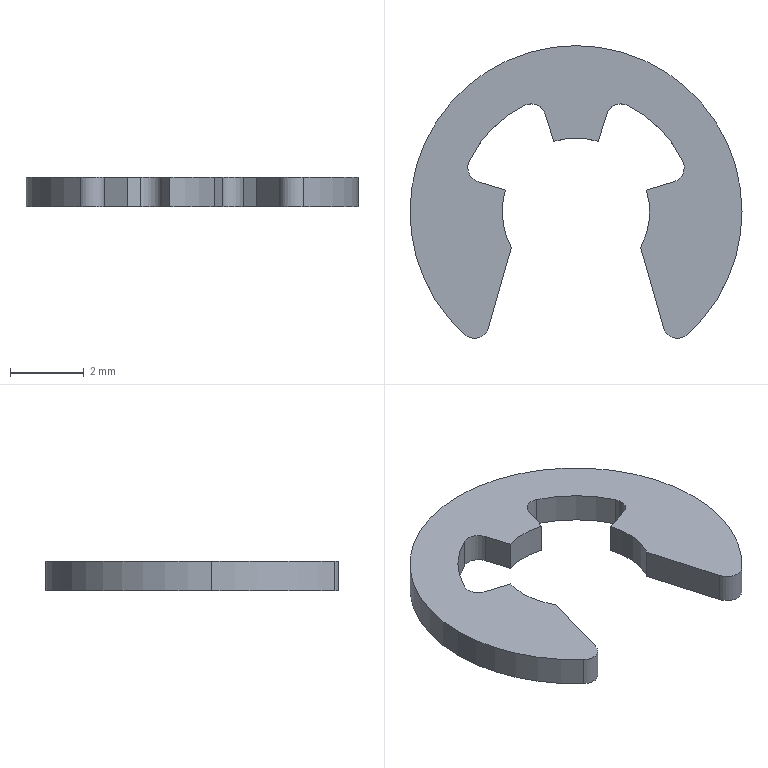Part | NX | features BREP 1 | 1 solid | 24 faces | box 9 x 7.933 x 0.8 mm | volume 26.47 mm3 | cylinder 16 | plane 8 | commonest cylinder face diameters 0.8 x7 4 x4 9 x3 6.4 x2
STEP:
#1=CARTESIAN_POINT('',(2.895,1.363,0.8));
#2=VERTEX_POINT('',#1);
#3=CARTESIAN_POINT('',(2.895,1.363,0.));
#4=VERTEX_POINT('',#3);
#5=CARTESIAN_POINT('',(2.895,1.363,0.8));
#6=DIRECTION('',(0.,0.,-1.));
#7=VECTOR('',#6,1000.);
#8=LINE('',#5,#7);
#9=EDGE_CURVE('',#2,#4,#8,.T.);
#10=ORIENTED_EDGE('',*,*,#9,.F.);
#11=CARTESIAN_POINT('',(1.388,2.883,0.8));
#12=VERTEX_POINT('',#11);
#13=CARTESIAN_POINT('',(0.,0.,0.8));
#14=DIRECTION('',(0.,0.,1.));
#15=DIRECTION('',(0.9047,0.426,0.));
#16=AXIS2_PLACEMENT_3D('',#13,#14,#15);
#17=CIRCLE('',#16,3.2);
#18=EDGE_CURVE('',#2,#12,#17,.T.);
#19=ORIENTED_EDGE('',*,*,#18,.T.);
#20=CARTESIAN_POINT('',(1.388,2.883,0.));
#21=VERTEX_POINT('',#20);
#22=CARTESIAN_POINT('',(1.388,2.883,0.));
#23=DIRECTION('',(0.,0.,1.));
#24=VECTOR('',#23,1000.);
#25=LINE('',#22,#24);
#26=EDGE_CURVE('',#21,#12,#25,.T.);
#27=ORIENTED_EDGE('',*,*,#26,.F.);
#28=CARTESIAN_POINT('',(0.,0.,0.));
#29=DIRECTION('',(0.,0.,-1.));
#30=DIRECTION('',(0.4339,0.901,0.));
#31=AXIS2_PLACEMENT_3D('',#28,#29,#30);
#32=CIRCLE('',#31,3.2);
#33=EDGE_CURVE('',#21,#4,#32,.T.);
#34=ORIENTED_EDGE('',*,*,#33,.T.);
#35=EDGE_LOOP('',(#10,#19,#27,#34));
#36=FACE_BOUND('',#35,.T.);
#37=CARTESIAN_POINT('',(0.,0.,0.8));
#38=DIRECTION('',(0.,0.,-1.));
#39=DIRECTION('',(-1.,0.,0.));
#40=AXIS2_PLACEMENT_3D('',#37,#38,#39);
#41=CYLINDRICAL_SURFACE('',#40,3.2);
#42=ADVANCED_FACE('',(#36),#41,.F.);
#43=CARTESIAN_POINT('',(0.8333,2.643,0.));
#44=VERTEX_POINT('',#43);
#45=CARTESIAN_POINT('',(1.215,2.523,0.));
#46=DIRECTION('',(0.,0.,-1.));
#47=DIRECTION('',(-0.9537,0.3007,0.));
#48=AXIS2_PLACEMENT_3D('',#45,#46,#47);
#49=CIRCLE('',#48,0.4);
#50=EDGE_CURVE('',#44,#21,#49,.T.);
#51=ORIENTED_EDGE('',*,*,#50,.F.);
#52=CARTESIAN_POINT('',(0.6014,1.907,0.));
#53=VERTEX_POINT('',#52);
#54=CARTESIAN_POINT('',(0.6014,1.907,0.));
#55=DIRECTION('',(0.3007,0.9537,0.));
#56=VECTOR('',#55,1000.);
#57=LINE('',#54,#56);
#58=EDGE_CURVE('',#53,#44,#57,.T.);
#59=ORIENTED_EDGE('',*,*,#58,.F.);
#60=CARTESIAN_POINT('',(-0.6014,1.907,0.));
#61=VERTEX_POINT('',#60);
#62=CARTESIAN_POINT('',(0.,0.,0.));
#63=DIRECTION('',(0.,0.,-1.));
#64=DIRECTION('',(-0.3007,0.9537,0.));
#65=AXIS2_PLACEMENT_3D('',#62,#63,#64);
#66=CIRCLE('',#65,2.);
#67=EDGE_CURVE('',#61,#53,#66,.T.);
#68=ORIENTED_EDGE('',*,*,#67,.F.);
#69=CARTESIAN_POINT('',(-0.8333,2.643,0.));
#70=VERTEX_POINT('',#69);
#71=CARTESIAN_POINT('',(-0.8333,2.643,0.));
#72=DIRECTION('',(0.3007,-0.9537,0.));
#73=VECTOR('',#72,1000.);
#74=LINE('',#71,#73);
#75=EDGE_CURVE('',#70,#61,#74,.T.);
#76=ORIENTED_EDGE('',*,*,#75,.F.);
#77=CARTESIAN_POINT('',(-1.388,2.883,0.));
#78=VERTEX_POINT('',#77);
#79=CARTESIAN_POINT('',(-1.215,2.523,0.));
#80=DIRECTION('',(0.,0.,-1.));
#81=DIRECTION('',(-0.4339,0.901,0.));
#82=AXIS2_PLACEMENT_3D('',#79,#80,#81);
#83=CIRCLE('',#82,0.4);
#84=EDGE_CURVE('',#78,#70,#83,.T.);
#85=ORIENTED_EDGE('',*,*,#84,.F.);
#86=CARTESIAN_POINT('',(-2.895,1.363,0.));
#87=VERTEX_POINT('',#86);
#88=CARTESIAN_POINT('',(0.,0.,0.));
#89=DIRECTION('',(0.,0.,-1.));
#90=DIRECTION('',(-0.9047,0.426,0.));
#91=AXIS2_PLACEMENT_3D('',#88,#89,#90);
#92=CIRCLE('',#91,3.2);
#93=EDGE_CURVE('',#87,#78,#92,.T.);
#94=ORIENTED_EDGE('',*,*,#93,.F.);
#95=CARTESIAN_POINT('',(-2.933,1.193,0.));
#96=VERTEX_POINT('',#95);
#97=CARTESIAN_POINT('',(-2.533,1.193,0.));
#98=DIRECTION('',(0.,0.,-1.));
#99=DIRECTION('',(-1.,0.,0.));
#100=AXIS2_PLACEMENT_3D('',#97,#98,#99);
#101=CIRCLE('',#100,0.4);
#102=EDGE_CURVE('',#96,#87,#101,.T.);
#103=ORIENTED_EDGE('',*,*,#102,.F.);
#104=CARTESIAN_POINT('',(-2.65,0.8102,0.));
#105=VERTEX_POINT('',#104);
#106=CARTESIAN_POINT('',(-2.533,1.193,0.));
#107=DIRECTION('',(0.,0.,-1.));
#108=DIRECTION('',(-1.,0.,0.));
#109=AXIS2_PLACEMENT_3D('',#106,#107,#108);
#110=CIRCLE('',#109,0.4);
#111=EDGE_CURVE('',#105,#96,#110,.T.);
#112=ORIENTED_EDGE('',*,*,#111,.F.);
#113=CARTESIAN_POINT('',(-1.913,0.5847,0.));
#114=VERTEX_POINT('',#113);
#115=CARTESIAN_POINT('',(-1.913,0.5847,0.));
#116=DIRECTION('',(-0.9563,0.2924,0.));
#117=VECTOR('',#116,1000.);
#118=LINE('',#115,#117);
#119=EDGE_CURVE('',#114,#105,#118,.T.);
#120=ORIENTED_EDGE('',*,*,#119,.F.);
#121=CARTESIAN_POINT('',(-2.,0.,0.));
#122=VERTEX_POINT('',#121);
#123=CARTESIAN_POINT('',(0.,0.,0.));
#124=DIRECTION('',(0.,0.,-1.));
#125=DIRECTION('',(-1.,0.,0.));
#126=AXIS2_PLACEMENT_3D('',#123,#124,#125);
#127=CIRCLE('',#126,2.);
#128=EDGE_CURVE('',#122,#114,#127,.T.);
#129=ORIENTED_EDGE('',*,*,#128,.F.);
#130=CARTESIAN_POINT('',(-1.75,-0.9682,0.));
#131=VERTEX_POINT('',#130);
#132=CARTESIAN_POINT('',(0.,0.,0.));
#133=DIRECTION('',(0.,0.,-1.));
#134=DIRECTION('',(-1.,0.,0.));
#135=AXIS2_PLACEMENT_3D('',#132,#133,#134);
#136=CIRCLE('',#135,2.);
#137=EDGE_CURVE('',#131,#122,#136,.T.);
#138=ORIENTED_EDGE('',*,*,#137,.F.);
#139=CARTESIAN_POINT('',(-2.374,-3.144,0.));
#140=VERTEX_POINT('',#139);
#141=CARTESIAN_POINT('',(-2.374,-3.144,0.));
#142=DIRECTION('',(0.2756,0.9613,0.));
#143=VECTOR('',#142,1000.);
#144=LINE('',#141,#143);
#145=EDGE_CURVE('',#140,#131,#144,.T.);
#146=ORIENTED_EDGE('',*,*,#145,.F.);
#147=CARTESIAN_POINT('',(-3.027,-3.329,0.));
#148=VERTEX_POINT('',#147);
#149=CARTESIAN_POINT('',(-2.758,-3.033,0.));
#150=DIRECTION('',(0.,0.,1.));
#151=DIRECTION('',(-0.6728,-0.7399,0.));
#152=AXIS2_PLACEMENT_3D('',#149,#150,#151);
#153=CIRCLE('',#152,0.4);
#154=EDGE_CURVE('',#148,#140,#153,.T.);
#155=ORIENTED_EDGE('',*,*,#154,.F.);
#156=CARTESIAN_POINT('',(-4.5,0.,0.));
#157=VERTEX_POINT('',#156);
#158=CARTESIAN_POINT('',(0.,0.,0.));
#159=DIRECTION('',(0.,0.,1.));
#160=DIRECTION('',(-1.,0.,0.));
#161=AXIS2_PLACEMENT_3D('',#158,#159,#160);
#162=CIRCLE('',#161,4.5);
#163=EDGE_CURVE('',#157,#148,#162,.T.);
#164=ORIENTED_EDGE('',*,*,#163,.F.);
#165=CARTESIAN_POINT('',(4.5,0.,0.));
#166=VERTEX_POINT('',#165);
#167=CARTESIAN_POINT('',(0.,0.,0.));
#168=DIRECTION('',(0.,0.,1.));
#169=DIRECTION('',(-1.,0.,0.));
#170=AXIS2_PLACEMENT_3D('',#167,#168,#169);
#171=CIRCLE('',#170,4.5);
#172=EDGE_CURVE('',#166,#157,#171,.T.);
#173=ORIENTED_EDGE('',*,*,#172,.F.);
#174=CARTESIAN_POINT('',(3.027,-3.329,0.));
#175=VERTEX_POINT('',#174);
#176=CARTESIAN_POINT('',(0.,0.,0.));
#177=DIRECTION('',(0.,0.,1.));
#178=DIRECTION('',(-1.,0.,0.));
#179=AXIS2_PLACEMENT_3D('',#176,#177,#178);
#180=CIRCLE('',#179,4.5);
#181=EDGE_CURVE('',#175,#166,#180,.T.);
#182=ORIENTED_EDGE('',*,*,#181,.F.);
#183=CARTESIAN_POINT('',(2.374,-3.144,0.));
#184=VERTEX_POINT('',#183);
#185=CARTESIAN_POINT('',(2.758,-3.033,0.));
#186=DIRECTION('',(0.,0.,1.));
#187=DIRECTION('',(-0.9613,-0.2756,0.));
#188=AXIS2_PLACEMENT_3D('',#185,#186,#187);
#189=CIRCLE('',#188,0.4);
#190=EDGE_CURVE('',#184,#175,#189,.T.);
#191=ORIENTED_EDGE('',*,*,#190,.F.);
#192=CARTESIAN_POINT('',(1.75,-0.9682,0.));
#193=VERTEX_POINT('',#192);
#194=CARTESIAN_POINT('',(1.75,-0.9682,0.));
#195=DIRECTION('',(0.2756,-0.9613,0.));
#196=VECTOR('',#195,1000.);
#197=LINE('',#194,#196);
#198=EDGE_CURVE('',#193,#184,#197,.T.);
#199=ORIENTED_EDGE('',*,*,#198,.F.);
#200=CARTESIAN_POINT('',(1.913,0.5847,0.));
#201=VERTEX_POINT('',#200);
#202=CARTESIAN_POINT('',(0.,0.,0.));
#203=DIRECTION('',(0.,0.,-1.));
#204=DIRECTION('',(1.,0.,0.));
#205=AXIS2_PLACEMENT_3D('',#202,#203,#204);
#206=CIRCLE('',#205,2.);
#207=EDGE_CURVE('',#201,#193,#206,.T.);
#208=ORIENTED_EDGE('',*,*,#207,.F.);
#209=CARTESIAN_POINT('',(2.65,0.8102,0.));
#210=VERTEX_POINT('',#209);
#211=CARTESIAN_POINT('',(2.65,0.8102,0.));
#212=DIRECTION('',(-0.9563,-0.2924,0.));
#213=VECTOR('',#212,1000.);
#214=LINE('',#211,#213);
#215=EDGE_CURVE('',#210,#201,#214,.T.);
#216=ORIENTED_EDGE('',*,*,#215,.F.);
#217=CARTESIAN_POINT('',(2.533,1.193,0.));
#218=DIRECTION('',(0.,0.,-1.));
#219=DIRECTION('',(1.,0.,0.));
#220=AXIS2_PLACEMENT_3D('',#217,#218,#219);
#221=CIRCLE('',#220,0.4);
#222=EDGE_CURVE('',#4,#210,#221,.T.);
#223=ORIENTED_EDGE('',*,*,#222,.F.);
#224=ORIENTED_EDGE('',*,*,#33,.F.);
#225=EDGE_LOOP('',(#51,#59,#68,#76,#85,#94,#103,#112,#120,#129,#138,#146,#155,#164,#173,#182,#191,#199,#208,#216,#223,#224));
#226=FACE_BOUND('',#225,.T.);
#227=CARTESIAN_POINT('',(0.,0.,0.));
#228=DIRECTION('',(0.,0.,1.));
#229=DIRECTION('',(1.,0.,0.));
#230=AXIS2_PLACEMENT_3D('',#227,#228,#229);
#231=PLANE('',#230);
#232=ADVANCED_FACE('',(#226),#231,.F.);
#233=ORIENTED_EDGE('',*,*,#222,.T.);
#234=CARTESIAN_POINT('',(2.65,0.8102,0.8));
#235=VERTEX_POINT('',#234);
#236=CARTESIAN_POINT('',(2.65,0.8102,0.8));
#237=DIRECTION('',(0.,0.,-1.));
#238=VECTOR('',#237,1000.);
#239=LINE('',#236,#238);
#240=EDGE_CURVE('',#235,#210,#239,.T.);
#241=ORIENTED_EDGE('',*,*,#240,.F.);
#242=CARTESIAN_POINT('',(2.533,1.193,0.8));
#243=DIRECTION('',(0.,0.,1.));
#244=DIRECTION('',(0.2924,-0.9563,0.));
#245=AXIS2_PLACEMENT_3D('',#242,#243,#244);
#246=CIRCLE('',#245,0.4);
#247=EDGE_CURVE('',#235,#2,#246,.T.);
#248=ORIENTED_EDGE('',*,*,#247,.T.);
#249=ORIENTED_EDGE('',*,*,#9,.T.);
#250=EDGE_LOOP('',(#233,#241,#248,#249));
#251=FACE_BOUND('',#250,.T.);
#252=CARTESIAN_POINT('',(2.533,1.193,0.8));
#253=DIRECTION('',(0.,0.,-1.));
#254=DIRECTION('',(-1.,0.,0.));
#255=AXIS2_PLACEMENT_3D('',#252,#253,#254);
#256=CYLINDRICAL_SURFACE('',#255,0.4);
#257=ADVANCED_FACE('',(#251),#256,.F.);
#258=ORIENTED_EDGE('',*,*,#18,.F.);
#259=ORIENTED_EDGE('',*,*,#247,.F.);
#260=CARTESIAN_POINT('',(1.913,0.5847,0.8));
#261=VERTEX_POINT('',#260);
#262=CARTESIAN_POINT('',(1.913,0.5847,0.8));
#263=DIRECTION('',(0.9563,0.2924,0.));
#264=VECTOR('',#263,1000.);
#265=LINE('',#262,#264);
#266=EDGE_CURVE('',#261,#235,#265,.T.);
#267=ORIENTED_EDGE('',*,*,#266,.F.);
#268=CARTESIAN_POINT('',(1.75,-0.9682,0.8));
#269=VERTEX_POINT('',#268);
#270=CARTESIAN_POINT('',(0.,0.,0.8));
#271=DIRECTION('',(0.,0.,1.));
#272=DIRECTION('',(1.,0.,0.));
#273=AXIS2_PLACEMENT_3D('',#270,#271,#272);
#274=CIRCLE('',#273,2.);
#275=EDGE_CURVE('',#269,#261,#274,.T.);
#276=ORIENTED_EDGE('',*,*,#275,.F.);
#277=CARTESIAN_POINT('',(2.374,-3.144,0.8));
#278=VERTEX_POINT('',#277);
#279=CARTESIAN_POINT('',(2.374,-3.144,0.8));
#280=DIRECTION('',(-0.2756,0.9613,0.));
#281=VECTOR('',#280,1000.);
#282=LINE('',#279,#281);
#283=EDGE_CURVE('',#278,#269,#282,.T.);
#284=ORIENTED_EDGE('',*,*,#283,.F.);
#285=CARTESIAN_POINT('',(3.027,-3.329,0.8));
#286=VERTEX_POINT('',#285);
#287=CARTESIAN_POINT('',(2.758,-3.033,0.8));
#288=DIRECTION('',(0.,0.,-1.));
#289=DIRECTION('',(0.6728,-0.7399,0.));
#290=AXIS2_PLACEMENT_3D('',#287,#288,#289);
#291=CIRCLE('',#290,0.4);
#292=EDGE_CURVE('',#286,#278,#291,.T.);
#293=ORIENTED_EDGE('',*,*,#292,.F.);
#294=CARTESIAN_POINT('',(4.5,0.,0.8));
#295=VERTEX_POINT('',#294);
#296=CARTESIAN_POINT('',(0.,0.,0.8));
#297=DIRECTION('',(0.,0.,-1.));
#298=DIRECTION('',(1.,0.,0.));
#299=AXIS2_PLACEMENT_3D('',#296,#297,#298);
#300=CIRCLE('',#299,4.5);
#301=EDGE_CURVE('',#295,#286,#300,.T.);
#302=ORIENTED_EDGE('',*,*,#301,.F.);
#303=CARTESIAN_POINT('',(-4.5,0.,0.8));
#304=VERTEX_POINT('',#303);
#305=CARTESIAN_POINT('',(0.,0.,0.8));
#306=DIRECTION('',(0.,0.,-1.));
#307=DIRECTION('',(1.,0.,0.));
#308=AXIS2_PLACEMENT_3D('',#305,#306,#307);
#309=CIRCLE('',#308,4.5);
#310=EDGE_CURVE('',#304,#295,#309,.T.);
#311=ORIENTED_EDGE('',*,*,#310,.F.);
#312=CARTESIAN_POINT('',(-3.027,-3.329,0.8));
#313=VERTEX_POINT('',#312);
#314=CARTESIAN_POINT('',(0.,0.,0.8));
#315=DIRECTION('',(0.,0.,-1.));
#316=DIRECTION('',(1.,0.,0.));
#317=AXIS2_PLACEMENT_3D('',#314,#315,#316);
#318=CIRCLE('',#317,4.5);
#319=EDGE_CURVE('',#313,#304,#318,.T.);
#320=ORIENTED_EDGE('',*,*,#319,.F.);
#321=CARTESIAN_POINT('',(-2.374,-3.144,0.8));
#322=VERTEX_POINT('',#321);
#323=CARTESIAN_POINT('',(-2.758,-3.033,0.8));
#324=DIRECTION('',(0.,0.,-1.));
#325=DIRECTION('',(0.9613,-0.2756,0.));
#326=AXIS2_PLACEMENT_3D('',#323,#324,#325);
#327=CIRCLE('',#326,0.4);
#328=EDGE_CURVE('',#322,#313,#327,.T.);
#329=ORIENTED_EDGE('',*,*,#328,.F.);
#330=CARTESIAN_POINT('',(-1.75,-0.9682,0.8));
#331=VERTEX_POINT('',#330);
#332=CARTESIAN_POINT('',(-1.75,-0.9682,0.8));
#333=DIRECTION('',(-0.2756,-0.9613,0.));
#334=VECTOR('',#333,1000.);
#335=LINE('',#332,#334);
#336=EDGE_CURVE('',#331,#322,#335,.T.);
#337=ORIENTED_EDGE('',*,*,#336,.F.);
#338=CARTESIAN_POINT('',(-2.,0.,0.8));
#339=VERTEX_POINT('',#338);
#340=CARTESIAN_POINT('',(0.,0.,0.8));
#341=DIRECTION('',(0.,0.,1.));
#342=DIRECTION('',(-1.,0.,0.));
#343=AXIS2_PLACEMENT_3D('',#340,#341,#342);
#344=CIRCLE('',#343,2.);
#345=EDGE_CURVE('',#339,#331,#344,.T.);
#346=ORIENTED_EDGE('',*,*,#345,.F.);
#347=CARTESIAN_POINT('',(-1.913,0.5847,0.8));
#348=VERTEX_POINT('',#347);
#349=CARTESIAN_POINT('',(0.,0.,0.8));
#350=DIRECTION('',(0.,0.,1.));
#351=DIRECTION('',(-1.,0.,0.));
#352=AXIS2_PLACEMENT_3D('',#349,#350,#351);
#353=CIRCLE('',#352,2.);
#354=EDGE_CURVE('',#348,#339,#353,.T.);
#355=ORIENTED_EDGE('',*,*,#354,.F.);
#356=CARTESIAN_POINT('',(-2.65,0.8102,0.8));
#357=VERTEX_POINT('',#356);
#358=CARTESIAN_POINT('',(-2.65,0.8102,0.8));
#359=DIRECTION('',(0.9563,-0.2924,0.));
#360=VECTOR('',#359,1000.);
#361=LINE('',#358,#360);
#362=EDGE_CURVE('',#357,#348,#361,.T.);
#363=ORIENTED_EDGE('',*,*,#362,.F.);
#364=CARTESIAN_POINT('',(-2.933,1.193,0.8));
#365=VERTEX_POINT('',#364);
#366=CARTESIAN_POINT('',(-2.533,1.193,0.8));
#367=DIRECTION('',(0.,0.,1.));
#368=DIRECTION('',(-1.,0.,0.));
#369=AXIS2_PLACEMENT_3D('',#366,#367,#368);
#370=CIRCLE('',#369,0.4);
#371=EDGE_CURVE('',#365,#357,#370,.T.);
#372=ORIENTED_EDGE('',*,*,#371,.F.);
#373=CARTESIAN_POINT('',(-2.895,1.363,0.8));
#374=VERTEX_POINT('',#373);
#375=CARTESIAN_POINT('',(-2.533,1.193,0.8));
#376=DIRECTION('',(0.,0.,1.));
#377=DIRECTION('',(-1.,0.,0.));
#378=AXIS2_PLACEMENT_3D('',#375,#376,#377);
#379=CIRCLE('',#378,0.4);
#380=EDGE_CURVE('',#374,#365,#379,.T.);
#381=ORIENTED_EDGE('',*,*,#380,.F.);
#382=CARTESIAN_POINT('',(-1.388,2.883,0.8));
#383=VERTEX_POINT('',#382);
#384=CARTESIAN_POINT('',(0.,0.,0.8));
#385=DIRECTION('',(0.,0.,1.));
#386=DIRECTION('',(-0.4339,0.901,0.));
#387=AXIS2_PLACEMENT_3D('',#384,#385,#386);
#388=CIRCLE('',#387,3.2);
#389=EDGE_CURVE('',#383,#374,#388,.T.);
#390=ORIENTED_EDGE('',*,*,#389,.F.);
#391=CARTESIAN_POINT('',(-0.8333,2.643,0.8));
#392=VERTEX_POINT('',#391);
#393=CARTESIAN_POINT('',(-1.215,2.523,0.8));
#394=DIRECTION('',(0.,0.,1.));
#395=DIRECTION('',(0.9537,0.3007,0.));
#396=AXIS2_PLACEMENT_3D('',#393,#394,#395);
#397=CIRCLE('',#396,0.4);
#398=EDGE_CURVE('',#392,#383,#397,.T.);
#399=ORIENTED_EDGE('',*,*,#398,.F.);
#400=CARTESIAN_POINT('',(-0.6014,1.907,0.8));
#401=VERTEX_POINT('',#400);
#402=CARTESIAN_POINT('',(-0.6014,1.907,0.8));
#403=DIRECTION('',(-0.3007,0.9537,0.));
#404=VECTOR('',#403,1000.);
#405=LINE('',#402,#404);
#406=EDGE_CURVE('',#401,#392,#405,.T.);
#407=ORIENTED_EDGE('',*,*,#406,.F.);
#408=CARTESIAN_POINT('',(0.6014,1.907,0.8));
#409=VERTEX_POINT('',#408);
#410=CARTESIAN_POINT('',(0.,0.,0.8));
#411=DIRECTION('',(0.,0.,1.));
#412=DIRECTION('',(0.3007,0.9537,0.));
#413=AXIS2_PLACEMENT_3D('',#410,#411,#412);
#414=CIRCLE('',#413,2.);
#415=EDGE_CURVE('',#409,#401,#414,.T.);
#416=ORIENTED_EDGE('',*,*,#415,.F.);
#417=CARTESIAN_POINT('',(0.8333,2.643,0.8));
#418=VERTEX_POINT('',#417);
#419=CARTESIAN_POINT('',(0.8333,2.643,0.8));
#420=DIRECTION('',(-0.3007,-0.9537,0.));
#421=VECTOR('',#420,1000.);
#422=LINE('',#419,#421);
#423=EDGE_CURVE('',#418,#409,#422,.T.);
#424=ORIENTED_EDGE('',*,*,#423,.F.);
#425=CARTESIAN_POINT('',(1.215,2.523,0.8));
#426=DIRECTION('',(0.,0.,1.));
#427=DIRECTION('',(0.4339,0.901,0.));
#428=AXIS2_PLACEMENT_3D('',#425,#426,#427);
#429=CIRCLE('',#428,0.4);
#430=EDGE_CURVE('',#12,#418,#429,.T.);
#431=ORIENTED_EDGE('',*,*,#430,.F.);
#432=EDGE_LOOP('',(#258,#259,#267,#276,#284,#293,#302,#311,#320,#329,#337,#346,#355,#363,#372,#381,#390,#399,#407,#416,#424,#431));
#433=FACE_BOUND('',#432,.T.);
#434=CARTESIAN_POINT('',(0.,0.,0.8));
#435=DIRECTION('',(0.,0.,1.));
#436=DIRECTION('',(1.,0.,0.));
#437=AXIS2_PLACEMENT_3D('',#434,#435,#436);
#438=PLANE('',#437);
#439=ADVANCED_FACE('',(#433),#438,.T.);
#440=ORIENTED_EDGE('',*,*,#26,.T.);
#441=ORIENTED_EDGE('',*,*,#430,.T.);
#442=CARTESIAN_POINT('',(0.8333,2.643,0.));
#443=DIRECTION('',(0.,0.,1.));
#444=VECTOR('',#443,1000.);
#445=LINE('',#442,#444);
#446=EDGE_CURVE('',#44,#418,#445,.T.);
#447=ORIENTED_EDGE('',*,*,#446,.F.);
#448=ORIENTED_EDGE('',*,*,#50,.T.);
#449=EDGE_LOOP('',(#440,#441,#447,#448));
#450=FACE_BOUND('',#449,.T.);
#451=CARTESIAN_POINT('',(1.215,2.523,0.8));
#452=DIRECTION('',(0.,0.,-1.));
#453=DIRECTION('',(-1.,0.,0.));
#454=AXIS2_PLACEMENT_3D('',#451,#452,#453);
#455=CYLINDRICAL_SURFACE('',#454,0.4);
#456=ADVANCED_FACE('',(#450),#455,.F.);
#457=ORIENTED_EDGE('',*,*,#446,.T.);
#458=ORIENTED_EDGE('',*,*,#423,.T.);
#459=CARTESIAN_POINT('',(0.6014,1.907,0.8));
#460=DIRECTION('',(0.,0.,-1.));
#461=VECTOR('',#460,1000.);
#462=LINE('',#459,#461);
#463=EDGE_CURVE('',#409,#53,#462,.T.);
#464=ORIENTED_EDGE('',*,*,#463,.T.);
#465=ORIENTED_EDGE('',*,*,#58,.T.);
#466=EDGE_LOOP('',(#457,#458,#464,#465));
#467=FACE_BOUND('',#466,.T.);
#468=CARTESIAN_POINT('',(0.,0.,0.8));
#469=DIRECTION('',(-0.9537,0.3007,0.));
#470=DIRECTION('',(0.,0.,1.));
#471=AXIS2_PLACEMENT_3D('',#468,#469,#470);
#472=PLANE('',#471);
#473=ADVANCED_FACE('',(#467),#472,.F.);
#474=ORIENTED_EDGE('',*,*,#463,.F.);
#475=ORIENTED_EDGE('',*,*,#415,.T.);
#476=CARTESIAN_POINT('',(-0.6014,1.907,0.));
#477=DIRECTION('',(0.,0.,1.));
#478=VECTOR('',#477,1000.);
#479=LINE('',#476,#478);
#480=EDGE_CURVE('',#61,#401,#479,.T.);
#481=ORIENTED_EDGE('',*,*,#480,.F.);
#482=ORIENTED_EDGE('',*,*,#67,.T.);
#483=EDGE_LOOP('',(#474,#475,#481,#482));
#484=FACE_BOUND('',#483,.T.);
#485=CARTESIAN_POINT('',(0.,0.,0.8));
#486=DIRECTION('',(0.,0.,-1.));
#487=DIRECTION('',(-1.,0.,0.));
#488=AXIS2_PLACEMENT_3D('',#485,#486,#487);
#489=CYLINDRICAL_SURFACE('',#488,2.);
#490=ADVANCED_FACE('',(#484),#489,.F.);
#491=ORIENTED_EDGE('',*,*,#480,.T.);
#492=ORIENTED_EDGE('',*,*,#406,.T.);
#493=CARTESIAN_POINT('',(-0.8333,2.643,0.8));
#494=DIRECTION('',(0.,0.,-1.));
#495=VECTOR('',#494,1000.);
#496=LINE('',#493,#495);
#497=EDGE_CURVE('',#392,#70,#496,.T.);
#498=ORIENTED_EDGE('',*,*,#497,.T.);
#499=ORIENTED_EDGE('',*,*,#75,.T.);
#500=EDGE_LOOP('',(#491,#492,#498,#499));
#501=FACE_BOUND('',#500,.T.);
#502=CARTESIAN_POINT('',(0.,0.,0.8));
#503=DIRECTION('',(-0.9537,-0.3007,0.));
#504=DIRECTION('',(-0.3007,0.9537,0.));
#505=AXIS2_PLACEMENT_3D('',#502,#503,#504);
#506=PLANE('',#505);
#507=ADVANCED_FACE('',(#501),#506,.T.);
#508=ORIENTED_EDGE('',*,*,#497,.F.);
#509=ORIENTED_EDGE('',*,*,#398,.T.);
#510=CARTESIAN_POINT('',(-1.388,2.883,0.8));
#511=DIRECTION('',(0.,0.,-1.));
#512=VECTOR('',#511,1000.);
#513=LINE('',#510,#512);
#514=EDGE_CURVE('',#383,#78,#513,.T.);
#515=ORIENTED_EDGE('',*,*,#514,.T.);
#516=ORIENTED_EDGE('',*,*,#84,.T.);
#517=EDGE_LOOP('',(#508,#509,#515,#516));
#518=FACE_BOUND('',#517,.T.);
#519=CARTESIAN_POINT('',(-1.215,2.523,0.8));
#520=DIRECTION('',(0.,0.,-1.));
#521=DIRECTION('',(-1.,0.,0.));
#522=AXIS2_PLACEMENT_3D('',#519,#520,#521);
#523=CYLINDRICAL_SURFACE('',#522,0.4);
#524=ADVANCED_FACE('',(#518),#523,.F.);
#525=ORIENTED_EDGE('',*,*,#514,.F.);
#526=ORIENTED_EDGE('',*,*,#389,.T.);
#527=CARTESIAN_POINT('',(-2.895,1.363,0.8));
#528=DIRECTION('',(0.,0.,-1.));
#529=VECTOR('',#528,1000.);
#530=LINE('',#527,#529);
#531=EDGE_CURVE('',#374,#87,#530,.T.);
#532=ORIENTED_EDGE('',*,*,#531,.T.);
#533=ORIENTED_EDGE('',*,*,#93,.T.);
#534=EDGE_LOOP('',(#525,#526,#532,#533));
#535=FACE_BOUND('',#534,.T.);
#536=CARTESIAN_POINT('',(0.,0.,0.8));
#537=DIRECTION('',(0.,0.,-1.));
#538=DIRECTION('',(-1.,0.,0.));
#539=AXIS2_PLACEMENT_3D('',#536,#537,#538);
#540=CYLINDRICAL_SURFACE('',#539,3.2);
#541=ADVANCED_FACE('',(#535),#540,.F.);
#542=CARTESIAN_POINT('',(-2.933,1.193,0.8));
#543=DIRECTION('',(0.,0.,-1.));
#544=VECTOR('',#543,1000.);
#545=LINE('',#542,#544);
#546=EDGE_CURVE('',#365,#96,#545,.T.);
#547=ORIENTED_EDGE('',*,*,#546,.F.);
#548=ORIENTED_EDGE('',*,*,#371,.T.);
#549=CARTESIAN_POINT('',(-2.65,0.8102,0.));
#550=DIRECTION('',(0.,0.,1.));
#551=VECTOR('',#550,1000.);
#552=LINE('',#549,#551);
#553=EDGE_CURVE('',#105,#357,#552,.T.);
#554=ORIENTED_EDGE('',*,*,#553,.F.);
#555=ORIENTED_EDGE('',*,*,#111,.T.);
#556=EDGE_LOOP('',(#547,#548,#554,#555));
#557=FACE_BOUND('',#556,.T.);
#558=CARTESIAN_POINT('',(-2.533,1.193,0.8));
#559=DIRECTION('',(0.,0.,-1.));
#560=DIRECTION('',(-1.,0.,0.));
#561=AXIS2_PLACEMENT_3D('',#558,#559,#560);
#562=CYLINDRICAL_SURFACE('',#561,0.4);
#563=ADVANCED_FACE('',(#557),#562,.F.);
#564=ORIENTED_EDGE('',*,*,#553,.T.);
#565=ORIENTED_EDGE('',*,*,#362,.T.);
#566=CARTESIAN_POINT('',(-1.913,0.5847,0.8));
#567=DIRECTION('',(0.,0.,-1.));
#568=VECTOR('',#567,1000.);
#569=LINE('',#566,#568);
#570=EDGE_CURVE('',#348,#114,#569,.T.);
#571=ORIENTED_EDGE('',*,*,#570,.T.);
#572=ORIENTED_EDGE('',*,*,#119,.T.);
#573=EDGE_LOOP('',(#564,#565,#571,#572));
#574=FACE_BOUND('',#573,.T.);
#575=CARTESIAN_POINT('',(0.,0.,0.8));
#576=DIRECTION('',(-0.2924,-0.9563,0.));
#577=DIRECTION('',(-0.9563,0.2924,0.));
#578=AXIS2_PLACEMENT_3D('',#575,#576,#577);
#579=PLANE('',#578);
#580=ADVANCED_FACE('',(#574),#579,.F.);
#581=CARTESIAN_POINT('',(-2.,0.,0.8));
#582=DIRECTION('',(0.,0.,-1.));
#583=VECTOR('',#582,1000.);
#584=LINE('',#581,#583);
#585=EDGE_CURVE('',#339,#122,#584,.T.);
#586=ORIENTED_EDGE('',*,*,#585,.F.);
#587=ORIENTED_EDGE('',*,*,#345,.T.);
#588=CARTESIAN_POINT('',(-1.75,-0.9682,0.));
#589=DIRECTION('',(0.,0.,1.));
#590=VECTOR('',#589,1000.);
#591=LINE('',#588,#590);
#592=EDGE_CURVE('',#131,#331,#591,.T.);
#593=ORIENTED_EDGE('',*,*,#592,.F.);
#594=ORIENTED_EDGE('',*,*,#137,.T.);
#595=EDGE_LOOP('',(#586,#587,#593,#594));
#596=FACE_BOUND('',#595,.T.);
#597=CARTESIAN_POINT('',(0.,0.,0.8));
#598=DIRECTION('',(0.,0.,-1.));
#599=DIRECTION('',(-1.,0.,0.));
#600=AXIS2_PLACEMENT_3D('',#597,#598,#599);
#601=CYLINDRICAL_SURFACE('',#600,2.);
#602=ADVANCED_FACE('',(#596),#601,.F.);
#603=ORIENTED_EDGE('',*,*,#592,.T.);
#604=ORIENTED_EDGE('',*,*,#336,.T.);
#605=CARTESIAN_POINT('',(-2.374,-3.144,0.8));
#606=DIRECTION('',(0.,0.,-1.));
#607=VECTOR('',#606,1000.);
#608=LINE('',#605,#607);
#609=EDGE_CURVE('',#322,#140,#608,.T.);
#610=ORIENTED_EDGE('',*,*,#609,.T.);
#611=ORIENTED_EDGE('',*,*,#145,.T.);
#612=EDGE_LOOP('',(#603,#604,#610,#611));
#613=FACE_BOUND('',#612,.T.);
#614=CARTESIAN_POINT('',(-1.36,0.3901,0.8));
#615=DIRECTION('',(0.9613,-0.2756,0.));
#616=DIRECTION('',(0.,0.,-1.));
#617=AXIS2_PLACEMENT_3D('',#614,#615,#616);
#618=PLANE('',#617);
#619=ADVANCED_FACE('',(#613),#618,.T.);
#620=ORIENTED_EDGE('',*,*,#609,.F.);
#621=ORIENTED_EDGE('',*,*,#328,.T.);
#622=CARTESIAN_POINT('',(-3.027,-3.329,0.8));
#623=DIRECTION('',(0.,0.,-1.));
#624=VECTOR('',#623,1000.);
#625=LINE('',#622,#624);
#626=EDGE_CURVE('',#313,#148,#625,.T.);
#627=ORIENTED_EDGE('',*,*,#626,.T.);
#628=ORIENTED_EDGE('',*,*,#154,.T.);
#629=EDGE_LOOP('',(#620,#621,#627,#628));
#630=FACE_BOUND('',#629,.T.);
#631=CARTESIAN_POINT('',(-2.758,-3.033,0.8));
#632=DIRECTION('',(0.,0.,-1.));
#633=DIRECTION('',(-1.,0.,0.));
#634=AXIS2_PLACEMENT_3D('',#631,#632,#633);
#635=CYLINDRICAL_SURFACE('',#634,0.4);
#636=ADVANCED_FACE('',(#630),#635,.T.);
#637=CARTESIAN_POINT('',(4.5,0.,0.8));
#638=DIRECTION('',(0.,0.,-1.));
#639=VECTOR('',#638,1000.);
#640=LINE('',#637,#639);
#641=EDGE_CURVE('',#295,#166,#640,.T.);
#642=ORIENTED_EDGE('',*,*,#641,.F.);
#643=ORIENTED_EDGE('',*,*,#301,.T.);
#644=CARTESIAN_POINT('',(3.027,-3.329,0.8));
#645=DIRECTION('',(0.,0.,-1.));
#646=VECTOR('',#645,1000.);
#647=LINE('',#644,#646);
#648=EDGE_CURVE('',#286,#175,#647,.T.);
#649=ORIENTED_EDGE('',*,*,#648,.T.);
#650=ORIENTED_EDGE('',*,*,#181,.T.);
#651=EDGE_LOOP('',(#642,#643,#649,#650));
#652=FACE_BOUND('',#651,.T.);
#653=CARTESIAN_POINT('',(0.,0.,0.8));
#654=DIRECTION('',(0.,0.,-1.));
#655=DIRECTION('',(-1.,0.,0.));
#656=AXIS2_PLACEMENT_3D('',#653,#654,#655);
#657=CYLINDRICAL_SURFACE('',#656,4.5);
#658=ADVANCED_FACE('',(#652),#657,.T.);
#659=ORIENTED_EDGE('',*,*,#648,.F.);
#660=ORIENTED_EDGE('',*,*,#292,.T.);
#661=CARTESIAN_POINT('',(2.374,-3.144,0.));
#662=DIRECTION('',(0.,0.,1.));
#663=VECTOR('',#662,1000.);
#664=LINE('',#661,#663);
#665=EDGE_CURVE('',#184,#278,#664,.T.);
#666=ORIENTED_EDGE('',*,*,#665,.F.);
#667=ORIENTED_EDGE('',*,*,#190,.T.);
#668=EDGE_LOOP('',(#659,#660,#666,#667));
#669=FACE_BOUND('',#668,.T.);
#670=CARTESIAN_POINT('',(2.758,-3.033,0.8));
#671=DIRECTION('',(0.,0.,-1.));
#672=DIRECTION('',(-1.,0.,0.));
#673=AXIS2_PLACEMENT_3D('',#670,#671,#672);
#674=CYLINDRICAL_SURFACE('',#673,0.4);
#675=ADVANCED_FACE('',(#669),#674,.T.);
#676=ORIENTED_EDGE('',*,*,#665,.T.);
#677=ORIENTED_EDGE('',*,*,#283,.T.);
#678=CARTESIAN_POINT('',(1.75,-0.9682,0.8));
#679=DIRECTION('',(0.,0.,-1.));
#680=VECTOR('',#679,1000.);
#681=LINE('',#678,#680);
#682=EDGE_CURVE('',#269,#193,#681,.T.);
#683=ORIENTED_EDGE('',*,*,#682,.T.);
#684=ORIENTED_EDGE('',*,*,#198,.T.);
#685=EDGE_LOOP('',(#676,#677,#683,#684));
#686=FACE_BOUND('',#685,.T.);
#687=CARTESIAN_POINT('',(1.36,0.3901,0.8));
#688=DIRECTION('',(0.9613,0.2756,0.));
#689=DIRECTION('',(0.,0.,-1.));
#690=AXIS2_PLACEMENT_3D('',#687,#688,#689);
#691=PLANE('',#690);
#692=ADVANCED_FACE('',(#686),#691,.F.);
#693=ORIENTED_EDGE('',*,*,#207,.T.);
#694=ORIENTED_EDGE('',*,*,#682,.F.);
#695=ORIENTED_EDGE('',*,*,#275,.T.);
#696=CARTESIAN_POINT('',(1.913,0.5847,0.));
#697=DIRECTION('',(0.,0.,1.));
#698=VECTOR('',#697,1000.);
#699=LINE('',#696,#698);
#700=EDGE_CURVE('',#201,#261,#699,.T.);
#701=ORIENTED_EDGE('',*,*,#700,.F.);
#702=EDGE_LOOP('',(#693,#694,#695,#701));
#703=FACE_BOUND('',#702,.T.);
#704=CARTESIAN_POINT('',(0.,0.,0.8));
#705=DIRECTION('',(0.,0.,-1.));
#706=DIRECTION('',(-1.,0.,0.));
#707=AXIS2_PLACEMENT_3D('',#704,#705,#706);
#708=CYLINDRICAL_SURFACE('',#707,2.);
#709=ADVANCED_FACE('',(#703),#708,.F.);
#710=ORIENTED_EDGE('',*,*,#700,.T.);
#711=ORIENTED_EDGE('',*,*,#266,.T.);
#712=ORIENTED_EDGE('',*,*,#240,.T.);
#713=ORIENTED_EDGE('',*,*,#215,.T.);
#714=EDGE_LOOP('',(#710,#711,#712,#713));
#715=FACE_BOUND('',#714,.T.);
#716=CARTESIAN_POINT('',(0.,0.,0.8));
#717=DIRECTION('',(-0.2924,0.9563,0.));
#718=DIRECTION('',(0.,0.,1.));
#719=AXIS2_PLACEMENT_3D('',#716,#717,#718);
#720=PLANE('',#719);
#721=ADVANCED_FACE('',(#715),#720,.T.);
#722=ORIENTED_EDGE('',*,*,#319,.T.);
#723=CARTESIAN_POINT('',(-4.5,0.,0.8));
#724=DIRECTION('',(0.,0.,-1.));
#725=VECTOR('',#724,1000.);
#726=LINE('',#723,#725);
#727=EDGE_CURVE('',#304,#157,#726,.T.);
#728=ORIENTED_EDGE('',*,*,#727,.T.);
#729=ORIENTED_EDGE('',*,*,#163,.T.);
#730=ORIENTED_EDGE('',*,*,#626,.F.);
#731=EDGE_LOOP('',(#722,#728,#729,#730));
#732=FACE_BOUND('',#731,.T.);
#733=CARTESIAN_POINT('',(0.,0.,0.8));
#734=DIRECTION('',(0.,0.,-1.));
#735=DIRECTION('',(-1.,0.,0.));
#736=AXIS2_PLACEMENT_3D('',#733,#734,#735);
#737=CYLINDRICAL_SURFACE('',#736,4.5);
#738=ADVANCED_FACE('',(#732),#737,.T.);
#739=ORIENTED_EDGE('',*,*,#310,.T.);
#740=ORIENTED_EDGE('',*,*,#641,.T.);
#741=ORIENTED_EDGE('',*,*,#172,.T.);
#742=ORIENTED_EDGE('',*,*,#727,.F.);
#743=EDGE_LOOP('',(#739,#740,#741,#742));
#744=FACE_BOUND('',#743,.T.);
#745=CARTESIAN_POINT('',(0.,0.,0.8));
#746=DIRECTION('',(0.,0.,-1.));
#747=DIRECTION('',(-1.,0.,0.));
#748=AXIS2_PLACEMENT_3D('',#745,#746,#747);
#749=CYLINDRICAL_SURFACE('',#748,4.5);
#750=ADVANCED_FACE('',(#744),#749,.T.);
#751=ORIENTED_EDGE('',*,*,#354,.T.);
#752=ORIENTED_EDGE('',*,*,#585,.T.);
#753=ORIENTED_EDGE('',*,*,#128,.T.);
#754=ORIENTED_EDGE('',*,*,#570,.F.);
#755=EDGE_LOOP('',(#751,#752,#753,#754));
#756=FACE_BOUND('',#755,.T.);
#757=CARTESIAN_POINT('',(0.,0.,0.8));
#758=DIRECTION('',(0.,0.,-1.));
#759=DIRECTION('',(-1.,0.,0.));
#760=AXIS2_PLACEMENT_3D('',#757,#758,#759);
#761=CYLINDRICAL_SURFACE('',#760,2.);
#762=ADVANCED_FACE('',(#756),#761,.F.);
#763=ORIENTED_EDGE('',*,*,#380,.T.);
#764=ORIENTED_EDGE('',*,*,#546,.T.);
#765=ORIENTED_EDGE('',*,*,#102,.T.);
#766=ORIENTED_EDGE('',*,*,#531,.F.);
#767=EDGE_LOOP('',(#763,#764,#765,#766));
#768=FACE_BOUND('',#767,.T.);
#769=CARTESIAN_POINT('',(-2.533,1.193,0.8));
#770=DIRECTION('',(0.,0.,-1.));
#771=DIRECTION('',(-1.,0.,0.));
#772=AXIS2_PLACEMENT_3D('',#769,#770,#771);
#773=CYLINDRICAL_SURFACE('',#772,0.4);
#774=ADVANCED_FACE('',(#768),#773,.F.);
#775=CLOSED_SHELL('',(#42,#232,#257,#439,#456,#473,#490,#507,#524,#541,#563,#580,#602,#619,#636,#658,#675,#692,#709,#721,#738,#750,#762,#774));
#776=MANIFOLD_SOLID_BREP('',#775);
#777=(LENGTH_UNIT()NAMED_UNIT(*)SI_UNIT(.MILLI.,.METRE.));
#778=UNCERTAINTY_MEASURE_WITH_UNIT(LENGTH_MEASURE(0.00001),#777,'','');
#779=(NAMED_UNIT(*)PLANE_ANGLE_UNIT()SI_UNIT($,.RADIAN.));
#780=(NAMED_UNIT(*)SI_UNIT($,.STERADIAN.)SOLID_ANGLE_UNIT());
#781=(GEOMETRIC_REPRESENTATION_CONTEXT(3)GLOBAL_UNCERTAINTY_ASSIGNED_CONTEXT((#778))GLOBAL_UNIT_ASSIGNED_CONTEXT((#777,#779,#780))REPRESENTATION_CONTEXT('',''));
#782=ADVANCED_BREP_SHAPE_REPRESENTATION('',(#776),#781);